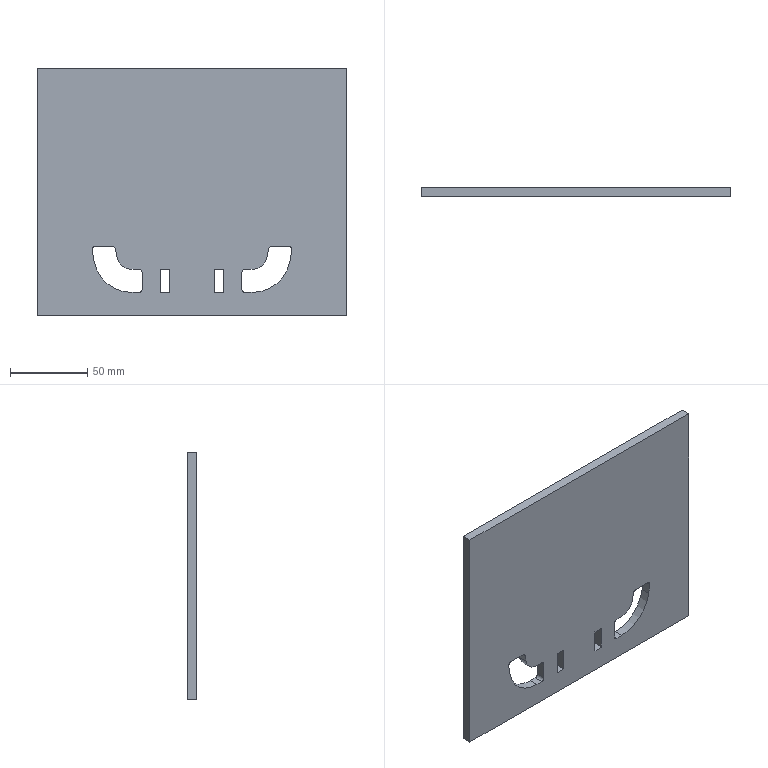Part | SolidWorks | features Cut 1, FlatPattern 1, ICE 1, SMBaseFlange 1, SheetMetal 1 | 1 solid | 38 faces | box 200 x 6 x 160 mm | volume 183961 mm3 | plane 26 | cylinder 12 | commonest cylinder face diameters 4 x8 20 x2 50 x2
STEP:
#1=CARTESIAN_POINT('',(100.,0.,80.));
#2=VERTEX_POINT('',#1);
#3=CARTESIAN_POINT('',(100.,0.,-80.));
#4=VERTEX_POINT('',#3);
#5=CARTESIAN_POINT('',(100.,0.,-80.));
#6=DIRECTION('',(0.,0.,-1.));
#7=VECTOR('',#6,1000.);
#8=LINE('',#5,#7);
#9=EDGE_CURVE('',#2,#4,#8,.T.);
#10=ORIENTED_EDGE('',*,*,#9,.T.);
#11=CARTESIAN_POINT('',(100.,6.,-80.));
#12=VERTEX_POINT('',#11);
#13=CARTESIAN_POINT('',(100.,6.,-80.));
#14=DIRECTION('',(0.,-1.,0.));
#15=VECTOR('',#14,1000.);
#16=LINE('',#13,#15);
#17=EDGE_CURVE('',#12,#4,#16,.T.);
#18=ORIENTED_EDGE('',*,*,#17,.F.);
#19=CARTESIAN_POINT('',(100.,6.,80.));
#20=VERTEX_POINT('',#19);
#21=CARTESIAN_POINT('',(100.,6.,-80.));
#22=DIRECTION('',(0.,0.,-1.));
#23=VECTOR('',#22,1000.);
#24=LINE('',#21,#23);
#25=EDGE_CURVE('',#20,#12,#24,.T.);
#26=ORIENTED_EDGE('',*,*,#25,.F.);
#27=CARTESIAN_POINT('',(100.,6.,80.));
#28=DIRECTION('',(0.,-1.,0.));
#29=VECTOR('',#28,1000.);
#30=LINE('',#27,#29);
#31=EDGE_CURVE('',#20,#2,#30,.T.);
#32=ORIENTED_EDGE('',*,*,#31,.T.);
#33=EDGE_LOOP('',(#10,#18,#26,#32));
#34=FACE_OUTER_BOUND('',#33,.T.);
#35=CARTESIAN_POINT('',(100.,6.,-80.));
#36=DIRECTION('',(-1.,0.,0.));
#37=DIRECTION('',(0.,0.,1.));
#38=AXIS2_PLACEMENT_3D('',#35,#36,#37);
#39=PLANE('',#38);
#40=ADVANCED_FACE('',(#34),#39,.F.);
#41=CARTESIAN_POINT('',(-100.,0.,-80.));
#42=VERTEX_POINT('',#41);
#43=CARTESIAN_POINT('',(-100.,0.,-80.));
#44=DIRECTION('',(-1.,0.,0.));
#45=VECTOR('',#44,1000.);
#46=LINE('',#43,#45);
#47=EDGE_CURVE('',#4,#42,#46,.T.);
#48=ORIENTED_EDGE('',*,*,#47,.T.);
#49=CARTESIAN_POINT('',(-100.,6.,-80.));
#50=VERTEX_POINT('',#49);
#51=CARTESIAN_POINT('',(-100.,6.,-80.));
#52=DIRECTION('',(0.,-1.,0.));
#53=VECTOR('',#52,1000.);
#54=LINE('',#51,#53);
#55=EDGE_CURVE('',#50,#42,#54,.T.);
#56=ORIENTED_EDGE('',*,*,#55,.F.);
#57=CARTESIAN_POINT('',(-100.,6.,-80.));
#58=DIRECTION('',(-1.,0.,0.));
#59=VECTOR('',#58,1000.);
#60=LINE('',#57,#59);
#61=EDGE_CURVE('',#12,#50,#60,.T.);
#62=ORIENTED_EDGE('',*,*,#61,.F.);
#63=ORIENTED_EDGE('',*,*,#17,.T.);
#64=EDGE_LOOP('',(#48,#56,#62,#63));
#65=FACE_OUTER_BOUND('',#64,.T.);
#66=CARTESIAN_POINT('',(-100.,6.,-80.));
#67=DIRECTION('',(0.,0.,1.));
#68=DIRECTION('',(1.,0.,0.));
#69=AXIS2_PLACEMENT_3D('',#66,#67,#68);
#70=PLANE('',#69);
#71=ADVANCED_FACE('',(#65),#70,.F.);
#72=CARTESIAN_POINT('',(-100.,0.,80.));
#73=VERTEX_POINT('',#72);
#74=CARTESIAN_POINT('',(-100.,0.,-80.));
#75=DIRECTION('',(0.,0.,1.));
#76=VECTOR('',#75,1000.);
#77=LINE('',#74,#76);
#78=EDGE_CURVE('',#42,#73,#77,.T.);
#79=ORIENTED_EDGE('',*,*,#78,.T.);
#80=CARTESIAN_POINT('',(-100.,6.,80.));
#81=VERTEX_POINT('',#80);
#82=CARTESIAN_POINT('',(-100.,6.,80.));
#83=DIRECTION('',(0.,-1.,0.));
#84=VECTOR('',#83,1000.);
#85=LINE('',#82,#84);
#86=EDGE_CURVE('',#81,#73,#85,.T.);
#87=ORIENTED_EDGE('',*,*,#86,.F.);
#88=CARTESIAN_POINT('',(-100.,6.,-80.));
#89=DIRECTION('',(0.,0.,1.));
#90=VECTOR('',#89,1000.);
#91=LINE('',#88,#90);
#92=EDGE_CURVE('',#50,#81,#91,.T.);
#93=ORIENTED_EDGE('',*,*,#92,.F.);
#94=ORIENTED_EDGE('',*,*,#55,.T.);
#95=EDGE_LOOP('',(#79,#87,#93,#94));
#96=FACE_OUTER_BOUND('',#95,.T.);
#97=CARTESIAN_POINT('',(-100.,6.,-80.));
#98=DIRECTION('',(1.,0.,0.));
#99=DIRECTION('',(0.,0.,-1.));
#100=AXIS2_PLACEMENT_3D('',#97,#98,#99);
#101=PLANE('',#100);
#102=ADVANCED_FACE('',(#96),#101,.F.);
#103=CARTESIAN_POINT('',(-100.,0.,80.));
#104=DIRECTION('',(1.,0.,0.));
#105=VECTOR('',#104,1000.);
#106=LINE('',#103,#105);
#107=EDGE_CURVE('',#73,#2,#106,.T.);
#108=ORIENTED_EDGE('',*,*,#107,.T.);
#109=ORIENTED_EDGE('',*,*,#31,.F.);
#110=CARTESIAN_POINT('',(-100.,6.,80.));
#111=DIRECTION('',(1.,0.,0.));
#112=VECTOR('',#111,1000.);
#113=LINE('',#110,#112);
#114=EDGE_CURVE('',#81,#20,#113,.T.);
#115=ORIENTED_EDGE('',*,*,#114,.F.);
#116=ORIENTED_EDGE('',*,*,#86,.T.);
#117=EDGE_LOOP('',(#108,#109,#115,#116));
#118=FACE_OUTER_BOUND('',#117,.T.);
#119=CARTESIAN_POINT('',(-100.,6.,80.));
#120=DIRECTION('',(0.,0.,-1.));
#121=DIRECTION('',(-1.,0.,0.));
#122=AXIS2_PLACEMENT_3D('',#119,#120,#121);
#123=PLANE('',#122);
#124=ADVANCED_FACE('',(#118),#123,.F.);
#125=CARTESIAN_POINT('',(-14.299,6.,-50.));
#126=VERTEX_POINT('',#125);
#127=CARTESIAN_POINT('',(-14.299,6.,-65.));
#128=VERTEX_POINT('',#127);
#129=CARTESIAN_POINT('',(-14.299,6.,-65.));
#130=DIRECTION('',(0.,0.,-1.));
#131=VECTOR('',#130,1000.);
#132=LINE('',#129,#131);
#133=EDGE_CURVE('',#126,#128,#132,.T.);
#134=ORIENTED_EDGE('',*,*,#133,.F.);
#135=CARTESIAN_POINT('',(-20.299,6.,-50.));
#136=VERTEX_POINT('',#135);
#137=CARTESIAN_POINT('',(-20.299,6.,-50.));
#138=DIRECTION('',(1.,0.,0.));
#139=VECTOR('',#138,1000.);
#140=LINE('',#137,#139);
#141=EDGE_CURVE('',#136,#126,#140,.T.);
#142=ORIENTED_EDGE('',*,*,#141,.F.);
#143=CARTESIAN_POINT('',(-20.299,6.,-65.));
#144=VERTEX_POINT('',#143);
#145=CARTESIAN_POINT('',(-20.299,6.,-65.));
#146=DIRECTION('',(0.,0.,1.));
#147=VECTOR('',#146,1000.);
#148=LINE('',#145,#147);
#149=EDGE_CURVE('',#144,#136,#148,.T.);
#150=ORIENTED_EDGE('',*,*,#149,.F.);
#151=CARTESIAN_POINT('',(-20.299,6.,-65.));
#152=DIRECTION('',(-1.,0.,0.));
#153=VECTOR('',#152,1000.);
#154=LINE('',#151,#153);
#155=EDGE_CURVE('',#128,#144,#154,.T.);
#156=ORIENTED_EDGE('',*,*,#155,.F.);
#157=EDGE_LOOP('',(#134,#142,#150,#156));
#158=FACE_BOUND('',#157,.T.);
#159=CARTESIAN_POINT('',(20.299,6.,-50.));
#160=VERTEX_POINT('',#159);
#161=CARTESIAN_POINT('',(20.299,6.,-65.));
#162=VERTEX_POINT('',#161);
#163=CARTESIAN_POINT('',(20.299,6.,-65.));
#164=DIRECTION('',(0.,0.,-1.));
#165=VECTOR('',#164,1000.);
#166=LINE('',#163,#165);
#167=EDGE_CURVE('',#160,#162,#166,.T.);
#168=ORIENTED_EDGE('',*,*,#167,.F.);
#169=CARTESIAN_POINT('',(14.299,6.,-50.));
#170=VERTEX_POINT('',#169);
#171=CARTESIAN_POINT('',(20.299,6.,-50.));
#172=DIRECTION('',(1.,0.,0.));
#173=VECTOR('',#172,1000.);
#174=LINE('',#171,#173);
#175=EDGE_CURVE('',#170,#160,#174,.T.);
#176=ORIENTED_EDGE('',*,*,#175,.F.);
#177=CARTESIAN_POINT('',(14.299,6.,-65.));
#178=VERTEX_POINT('',#177);
#179=CARTESIAN_POINT('',(14.299,6.,-65.));
#180=DIRECTION('',(0.,0.,1.));
#181=VECTOR('',#180,1000.);
#182=LINE('',#179,#181);
#183=EDGE_CURVE('',#178,#170,#182,.T.);
#184=ORIENTED_EDGE('',*,*,#183,.F.);
#185=CARTESIAN_POINT('',(20.299,6.,-65.));
#186=DIRECTION('',(-1.,0.,0.));
#187=VECTOR('',#186,1000.);
#188=LINE('',#185,#187);
#189=EDGE_CURVE('',#162,#178,#188,.T.);
#190=ORIENTED_EDGE('',*,*,#189,.F.);
#191=EDGE_LOOP('',(#168,#176,#184,#190));
#192=FACE_BOUND('',#191,.T.);
#193=CARTESIAN_POINT('',(-38.819,6.,-65.));
#194=VERTEX_POINT('',#193);
#195=CARTESIAN_POINT('',(-63.483,6.,-44.083));
#196=VERTEX_POINT('',#195);
#197=CARTESIAN_POINT('',(-38.819,6.,-40.));
#198=DIRECTION('',(0.,1.,0.));
#199=DIRECTION('',(0.,0.,1.));
#200=AXIS2_PLACEMENT_3D('',#197,#198,#199);
#201=CIRCLE('',#200,25.);
#202=EDGE_CURVE('',#194,#196,#201,.T.);
#203=ORIENTED_EDGE('',*,*,#202,.F.);
#204=CARTESIAN_POINT('',(-34.299,6.,-65.));
#205=VERTEX_POINT('',#204);
#206=CARTESIAN_POINT('',(-34.299,6.,-65.));
#207=DIRECTION('',(-1.,0.,0.));
#208=VECTOR('',#207,1000.);
#209=LINE('',#206,#208);
#210=EDGE_CURVE('',#205,#194,#209,.T.);
#211=ORIENTED_EDGE('',*,*,#210,.F.);
#212=CARTESIAN_POINT('',(-32.299,6.,-63.));
#213=VERTEX_POINT('',#212);
#214=CARTESIAN_POINT('',(-34.299,6.,-63.));
#215=DIRECTION('',(0.,1.,0.));
#216=DIRECTION('',(0.,0.,1.));
#217=AXIS2_PLACEMENT_3D('',#214,#215,#216);
#218=CIRCLE('',#217,2.);
#219=EDGE_CURVE('',#213,#205,#218,.T.);
#220=ORIENTED_EDGE('',*,*,#219,.F.);
#221=CARTESIAN_POINT('',(-32.299,6.,-52.));
#222=VERTEX_POINT('',#221);
#223=CARTESIAN_POINT('',(-32.299,6.,-52.));
#224=DIRECTION('',(0.,0.,-1.));
#225=VECTOR('',#224,1000.);
#226=LINE('',#223,#225);
#227=EDGE_CURVE('',#222,#213,#226,.T.);
#228=ORIENTED_EDGE('',*,*,#227,.F.);
#229=CARTESIAN_POINT('',(-34.299,6.,-50.));
#230=VERTEX_POINT('',#229);
#231=CARTESIAN_POINT('',(-34.299,6.,-52.));
#232=DIRECTION('',(0.,1.,0.));
#233=DIRECTION('',(0.,0.,1.));
#234=AXIS2_PLACEMENT_3D('',#231,#232,#233);
#235=CIRCLE('',#234,2.);
#236=EDGE_CURVE('',#230,#222,#235,.T.);
#237=ORIENTED_EDGE('',*,*,#236,.F.);
#238=CARTESIAN_POINT('',(-38.819,6.,-50.));
#239=VERTEX_POINT('',#238);
#240=CARTESIAN_POINT('',(-38.819,6.,-50.));
#241=DIRECTION('',(1.,0.,0.));
#242=VECTOR('',#241,1000.);
#243=LINE('',#240,#242);
#244=EDGE_CURVE('',#239,#230,#243,.T.);
#245=ORIENTED_EDGE('',*,*,#244,.F.);
#246=CARTESIAN_POINT('',(-48.685,6.,-41.633));
#247=VERTEX_POINT('',#246);
#248=CARTESIAN_POINT('',(-38.819,6.,-40.));
#249=DIRECTION('',(0.,-1.,0.));
#250=DIRECTION('',(0.,0.,1.));
#251=AXIS2_PLACEMENT_3D('',#248,#249,#250);
#252=CIRCLE('',#251,10.);
#253=EDGE_CURVE('',#247,#239,#252,.T.);
#254=ORIENTED_EDGE('',*,*,#253,.F.);
#255=CARTESIAN_POINT('',(-49.472,6.,-36.875));
#256=VERTEX_POINT('',#255);
#257=CARTESIAN_POINT('',(-49.472,6.,-36.875));
#258=DIRECTION('',(0.1633,0.,-0.9866));
#259=VECTOR('',#258,1000.);
#260=LINE('',#257,#259);
#261=EDGE_CURVE('',#256,#247,#260,.T.);
#262=ORIENTED_EDGE('',*,*,#261,.F.);
#263=CARTESIAN_POINT('',(-51.446,6.,-35.201));
#264=VERTEX_POINT('',#263);
#265=CARTESIAN_POINT('',(-51.446,6.,-37.201));
#266=DIRECTION('',(0.,1.,0.));
#267=DIRECTION('',(0.,0.,1.));
#268=AXIS2_PLACEMENT_3D('',#265,#266,#267);
#269=CIRCLE('',#268,2.);
#270=EDGE_CURVE('',#264,#256,#269,.T.);
#271=ORIENTED_EDGE('',*,*,#270,.F.);
#272=CARTESIAN_POINT('',(-62.595,6.,-35.201));
#273=VERTEX_POINT('',#272);
#274=CARTESIAN_POINT('',(-62.595,6.,-35.201));
#275=DIRECTION('',(1.,0.,0.));
#276=VECTOR('',#275,1000.);
#277=LINE('',#274,#276);
#278=EDGE_CURVE('',#273,#264,#277,.T.);
#279=ORIENTED_EDGE('',*,*,#278,.F.);
#280=CARTESIAN_POINT('',(-64.568,6.,-37.528));
#281=VERTEX_POINT('',#280);
#282=CARTESIAN_POINT('',(-62.595,6.,-37.201));
#283=DIRECTION('',(0.,1.,0.));
#284=DIRECTION('',(0.,0.,1.));
#285=AXIS2_PLACEMENT_3D('',#282,#283,#284);
#286=CIRCLE('',#285,2.);
#287=EDGE_CURVE('',#281,#273,#286,.T.);
#288=ORIENTED_EDGE('',*,*,#287,.F.);
#289=CARTESIAN_POINT('',(-63.483,6.,-44.083));
#290=DIRECTION('',(-0.1633,0.,0.9866));
#291=VECTOR('',#290,1000.);
#292=LINE('',#289,#291);
#293=EDGE_CURVE('',#196,#281,#292,.T.);
#294=ORIENTED_EDGE('',*,*,#293,.F.);
#295=EDGE_LOOP('',(#203,#211,#220,#228,#237,#245,#254,#262,#271,#279,#288,#294));
#296=FACE_BOUND('',#295,.T.);
#297=CARTESIAN_POINT('',(49.472,6.,-36.875));
#298=VERTEX_POINT('',#297);
#299=CARTESIAN_POINT('',(51.446,6.,-35.201));
#300=VERTEX_POINT('',#299);
#301=CARTESIAN_POINT('',(51.446,6.,-37.201));
#302=DIRECTION('',(0.,1.,0.));
#303=DIRECTION('',(0.,0.,1.));
#304=AXIS2_PLACEMENT_3D('',#301,#302,#303);
#305=CIRCLE('',#304,2.);
#306=EDGE_CURVE('',#298,#300,#305,.T.);
#307=ORIENTED_EDGE('',*,*,#306,.F.);
#308=CARTESIAN_POINT('',(48.685,6.,-41.633));
#309=VERTEX_POINT('',#308);
#310=CARTESIAN_POINT('',(48.685,6.,-41.633));
#311=DIRECTION('',(0.1633,0.,0.9866));
#312=VECTOR('',#311,1000.);
#313=LINE('',#310,#312);
#314=EDGE_CURVE('',#309,#298,#313,.T.);
#315=ORIENTED_EDGE('',*,*,#314,.F.);
#316=CARTESIAN_POINT('',(38.819,6.,-50.));
#317=VERTEX_POINT('',#316);
#318=CARTESIAN_POINT('',(38.819,6.,-40.));
#319=DIRECTION('',(0.,-1.,0.));
#320=DIRECTION('',(0.,0.,1.));
#321=AXIS2_PLACEMENT_3D('',#318,#319,#320);
#322=CIRCLE('',#321,10.);
#323=EDGE_CURVE('',#317,#309,#322,.T.);
#324=ORIENTED_EDGE('',*,*,#323,.F.);
#325=CARTESIAN_POINT('',(34.299,6.,-50.));
#326=VERTEX_POINT('',#325);
#327=CARTESIAN_POINT('',(34.299,6.,-50.));
#328=DIRECTION('',(1.,0.,0.));
#329=VECTOR('',#328,1000.);
#330=LINE('',#327,#329);
#331=EDGE_CURVE('',#326,#317,#330,.T.);
#332=ORIENTED_EDGE('',*,*,#331,.F.);
#333=CARTESIAN_POINT('',(32.299,6.,-52.));
#334=VERTEX_POINT('',#333);
#335=CARTESIAN_POINT('',(34.299,6.,-52.));
#336=DIRECTION('',(0.,1.,0.));
#337=DIRECTION('',(0.,0.,1.));
#338=AXIS2_PLACEMENT_3D('',#335,#336,#337);
#339=CIRCLE('',#338,2.);
#340=EDGE_CURVE('',#334,#326,#339,.T.);
#341=ORIENTED_EDGE('',*,*,#340,.F.);
#342=CARTESIAN_POINT('',(32.299,6.,-63.));
#343=VERTEX_POINT('',#342);
#344=CARTESIAN_POINT('',(32.299,6.,-63.));
#345=DIRECTION('',(0.,0.,1.));
#346=VECTOR('',#345,1000.);
#347=LINE('',#344,#346);
#348=EDGE_CURVE('',#343,#334,#347,.T.);
#349=ORIENTED_EDGE('',*,*,#348,.F.);
#350=CARTESIAN_POINT('',(34.299,6.,-65.));
#351=VERTEX_POINT('',#350);
#352=CARTESIAN_POINT('',(34.299,6.,-63.));
#353=DIRECTION('',(0.,1.,0.));
#354=DIRECTION('',(0.,0.,1.));
#355=AXIS2_PLACEMENT_3D('',#352,#353,#354);
#356=CIRCLE('',#355,2.);
#357=EDGE_CURVE('',#351,#343,#356,.T.);
#358=ORIENTED_EDGE('',*,*,#357,.F.);
#359=CARTESIAN_POINT('',(38.819,6.,-65.));
#360=VERTEX_POINT('',#359);
#361=CARTESIAN_POINT('',(38.819,6.,-65.));
#362=DIRECTION('',(-1.,0.,0.));
#363=VECTOR('',#362,1000.);
#364=LINE('',#361,#363);
#365=EDGE_CURVE('',#360,#351,#364,.T.);
#366=ORIENTED_EDGE('',*,*,#365,.F.);
#367=CARTESIAN_POINT('',(63.483,6.,-44.083));
#368=VERTEX_POINT('',#367);
#369=CARTESIAN_POINT('',(38.819,6.,-40.));
#370=DIRECTION('',(0.,1.,0.));
#371=DIRECTION('',(0.,0.,1.));
#372=AXIS2_PLACEMENT_3D('',#369,#370,#371);
#373=CIRCLE('',#372,25.);
#374=EDGE_CURVE('',#368,#360,#373,.T.);
#375=ORIENTED_EDGE('',*,*,#374,.F.);
#376=CARTESIAN_POINT('',(64.568,6.,-37.528));
#377=VERTEX_POINT('',#376);
#378=CARTESIAN_POINT('',(64.568,6.,-37.528));
#379=DIRECTION('',(-0.1633,0.,-0.9866));
#380=VECTOR('',#379,1000.);
#381=LINE('',#378,#380);
#382=EDGE_CURVE('',#377,#368,#381,.T.);
#383=ORIENTED_EDGE('',*,*,#382,.F.);
#384=CARTESIAN_POINT('',(62.595,6.,-35.201));
#385=VERTEX_POINT('',#384);
#386=CARTESIAN_POINT('',(62.595,6.,-37.201));
#387=DIRECTION('',(0.,1.,0.));
#388=DIRECTION('',(0.,0.,1.));
#389=AXIS2_PLACEMENT_3D('',#386,#387,#388);
#390=CIRCLE('',#389,2.);
#391=EDGE_CURVE('',#385,#377,#390,.T.);
#392=ORIENTED_EDGE('',*,*,#391,.F.);
#393=CARTESIAN_POINT('',(51.446,6.,-35.201));
#394=DIRECTION('',(1.,0.,0.));
#395=VECTOR('',#394,1000.);
#396=LINE('',#393,#395);
#397=EDGE_CURVE('',#300,#385,#396,.T.);
#398=ORIENTED_EDGE('',*,*,#397,.F.);
#399=EDGE_LOOP('',(#307,#315,#324,#332,#341,#349,#358,#366,#375,#383,#392,#398));
#400=FACE_BOUND('',#399,.T.);
#401=ORIENTED_EDGE('',*,*,#25,.T.);
#402=ORIENTED_EDGE('',*,*,#61,.T.);
#403=ORIENTED_EDGE('',*,*,#92,.T.);
#404=ORIENTED_EDGE('',*,*,#114,.T.);
#405=EDGE_LOOP('',(#401,#402,#403,#404));
#406=FACE_OUTER_BOUND('',#405,.T.);
#407=CARTESIAN_POINT('',(0.,6.,0.));
#408=DIRECTION('',(0.,1.,0.));
#409=DIRECTION('',(0.,0.,1.));
#410=AXIS2_PLACEMENT_3D('',#407,#408,#409);
#411=PLANE('',#410);
#412=ADVANCED_FACE('',(#158,#192,#296,#400,#406),#411,.T.);
#413=CARTESIAN_POINT('',(-20.299,0.,-50.));
#414=VERTEX_POINT('',#413);
#415=CARTESIAN_POINT('',(-14.299,0.,-50.));
#416=VERTEX_POINT('',#415);
#417=CARTESIAN_POINT('',(-20.299,0.,-50.));
#418=DIRECTION('',(1.,0.,0.));
#419=VECTOR('',#418,1000.);
#420=LINE('',#417,#419);
#421=EDGE_CURVE('',#414,#416,#420,.T.);
#422=ORIENTED_EDGE('',*,*,#421,.T.);
#423=CARTESIAN_POINT('',(-14.299,0.,-65.));
#424=VERTEX_POINT('',#423);
#425=CARTESIAN_POINT('',(-14.299,0.,-65.));
#426=DIRECTION('',(0.,0.,-1.));
#427=VECTOR('',#426,1000.);
#428=LINE('',#425,#427);
#429=EDGE_CURVE('',#416,#424,#428,.T.);
#430=ORIENTED_EDGE('',*,*,#429,.T.);
#431=CARTESIAN_POINT('',(-20.299,0.,-65.));
#432=VERTEX_POINT('',#431);
#433=CARTESIAN_POINT('',(-20.299,0.,-65.));
#434=DIRECTION('',(-1.,0.,0.));
#435=VECTOR('',#434,1000.);
#436=LINE('',#433,#435);
#437=EDGE_CURVE('',#424,#432,#436,.T.);
#438=ORIENTED_EDGE('',*,*,#437,.T.);
#439=CARTESIAN_POINT('',(-20.299,0.,-65.));
#440=DIRECTION('',(0.,0.,1.));
#441=VECTOR('',#440,1000.);
#442=LINE('',#439,#441);
#443=EDGE_CURVE('',#432,#414,#442,.T.);
#444=ORIENTED_EDGE('',*,*,#443,.T.);
#445=EDGE_LOOP('',(#422,#430,#438,#444));
#446=FACE_BOUND('',#445,.T.);
#447=CARTESIAN_POINT('',(14.299,0.,-50.));
#448=VERTEX_POINT('',#447);
#449=CARTESIAN_POINT('',(20.299,0.,-50.));
#450=VERTEX_POINT('',#449);
#451=CARTESIAN_POINT('',(20.299,0.,-50.));
#452=DIRECTION('',(1.,0.,0.));
#453=VECTOR('',#452,1000.);
#454=LINE('',#451,#453);
#455=EDGE_CURVE('',#448,#450,#454,.T.);
#456=ORIENTED_EDGE('',*,*,#455,.T.);
#457=CARTESIAN_POINT('',(20.299,0.,-65.));
#458=VERTEX_POINT('',#457);
#459=CARTESIAN_POINT('',(20.299,0.,-65.));
#460=DIRECTION('',(0.,0.,-1.));
#461=VECTOR('',#460,1000.);
#462=LINE('',#459,#461);
#463=EDGE_CURVE('',#450,#458,#462,.T.);
#464=ORIENTED_EDGE('',*,*,#463,.T.);
#465=CARTESIAN_POINT('',(14.299,0.,-65.));
#466=VERTEX_POINT('',#465);
#467=CARTESIAN_POINT('',(20.299,0.,-65.));
#468=DIRECTION('',(-1.,0.,0.));
#469=VECTOR('',#468,1000.);
#470=LINE('',#467,#469);
#471=EDGE_CURVE('',#458,#466,#470,.T.);
#472=ORIENTED_EDGE('',*,*,#471,.T.);
#473=CARTESIAN_POINT('',(14.299,0.,-65.));
#474=DIRECTION('',(0.,0.,1.));
#475=VECTOR('',#474,1000.);
#476=LINE('',#473,#475);
#477=EDGE_CURVE('',#466,#448,#476,.T.);
#478=ORIENTED_EDGE('',*,*,#477,.T.);
#479=EDGE_LOOP('',(#456,#464,#472,#478));
#480=FACE_BOUND('',#479,.T.);
#481=CARTESIAN_POINT('',(-34.299,0.,-65.));
#482=VERTEX_POINT('',#481);
#483=CARTESIAN_POINT('',(-38.819,0.,-65.));
#484=VERTEX_POINT('',#483);
#485=CARTESIAN_POINT('',(-34.299,0.,-65.));
#486=DIRECTION('',(-1.,0.,0.));
#487=VECTOR('',#486,1000.);
#488=LINE('',#485,#487);
#489=EDGE_CURVE('',#482,#484,#488,.T.);
#490=ORIENTED_EDGE('',*,*,#489,.T.);
#491=CARTESIAN_POINT('',(-63.483,0.,-44.083));
#492=VERTEX_POINT('',#491);
#493=CARTESIAN_POINT('',(-38.819,0.,-40.));
#494=DIRECTION('',(0.,1.,0.));
#495=DIRECTION('',(0.,0.,1.));
#496=AXIS2_PLACEMENT_3D('',#493,#494,#495);
#497=CIRCLE('',#496,25.);
#498=EDGE_CURVE('',#484,#492,#497,.T.);
#499=ORIENTED_EDGE('',*,*,#498,.T.);
#500=CARTESIAN_POINT('',(-64.568,0.,-37.528));
#501=VERTEX_POINT('',#500);
#502=CARTESIAN_POINT('',(-63.483,0.,-44.083));
#503=DIRECTION('',(-0.1633,0.,0.9866));
#504=VECTOR('',#503,1000.);
#505=LINE('',#502,#504);
#506=EDGE_CURVE('',#492,#501,#505,.T.);
#507=ORIENTED_EDGE('',*,*,#506,.T.);
#508=CARTESIAN_POINT('',(-62.595,0.,-35.201));
#509=VERTEX_POINT('',#508);
#510=CARTESIAN_POINT('',(-62.595,0.,-37.201));
#511=DIRECTION('',(0.,1.,0.));
#512=DIRECTION('',(0.,0.,1.));
#513=AXIS2_PLACEMENT_3D('',#510,#511,#512);
#514=CIRCLE('',#513,2.);
#515=EDGE_CURVE('',#501,#509,#514,.T.);
#516=ORIENTED_EDGE('',*,*,#515,.T.);
#517=CARTESIAN_POINT('',(-51.446,0.,-35.201));
#518=VERTEX_POINT('',#517);
#519=CARTESIAN_POINT('',(-62.595,0.,-35.201));
#520=DIRECTION('',(1.,0.,0.));
#521=VECTOR('',#520,1000.);
#522=LINE('',#519,#521);
#523=EDGE_CURVE('',#509,#518,#522,.T.);
#524=ORIENTED_EDGE('',*,*,#523,.T.);
#525=CARTESIAN_POINT('',(-49.472,0.,-36.875));
#526=VERTEX_POINT('',#525);
#527=CARTESIAN_POINT('',(-51.446,0.,-37.201));
#528=DIRECTION('',(0.,1.,0.));
#529=DIRECTION('',(0.,0.,1.));
#530=AXIS2_PLACEMENT_3D('',#527,#528,#529);
#531=CIRCLE('',#530,2.);
#532=EDGE_CURVE('',#518,#526,#531,.T.);
#533=ORIENTED_EDGE('',*,*,#532,.T.);
#534=CARTESIAN_POINT('',(-48.685,0.,-41.633));
#535=VERTEX_POINT('',#534);
#536=CARTESIAN_POINT('',(-49.472,0.,-36.875));
#537=DIRECTION('',(0.1633,0.,-0.9866));
#538=VECTOR('',#537,1000.);
#539=LINE('',#536,#538);
#540=EDGE_CURVE('',#526,#535,#539,.T.);
#541=ORIENTED_EDGE('',*,*,#540,.T.);
#542=CARTESIAN_POINT('',(-38.819,0.,-50.));
#543=VERTEX_POINT('',#542);
#544=CARTESIAN_POINT('',(-38.819,0.,-40.));
#545=DIRECTION('',(0.,-1.,0.));
#546=DIRECTION('',(0.,0.,1.));
#547=AXIS2_PLACEMENT_3D('',#544,#545,#546);
#548=CIRCLE('',#547,10.);
#549=EDGE_CURVE('',#535,#543,#548,.T.);
#550=ORIENTED_EDGE('',*,*,#549,.T.);
#551=CARTESIAN_POINT('',(-34.299,0.,-50.));
#552=VERTEX_POINT('',#551);
#553=CARTESIAN_POINT('',(-38.819,0.,-50.));
#554=DIRECTION('',(1.,0.,0.));
#555=VECTOR('',#554,1000.);
#556=LINE('',#553,#555);
#557=EDGE_CURVE('',#543,#552,#556,.T.);
#558=ORIENTED_EDGE('',*,*,#557,.T.);
#559=CARTESIAN_POINT('',(-32.299,0.,-52.));
#560=VERTEX_POINT('',#559);
#561=CARTESIAN_POINT('',(-34.299,0.,-52.));
#562=DIRECTION('',(0.,1.,0.));
#563=DIRECTION('',(0.,0.,1.));
#564=AXIS2_PLACEMENT_3D('',#561,#562,#563);
#565=CIRCLE('',#564,2.);
#566=EDGE_CURVE('',#552,#560,#565,.T.);
#567=ORIENTED_EDGE('',*,*,#566,.T.);
#568=CARTESIAN_POINT('',(-32.299,0.,-63.));
#569=VERTEX_POINT('',#568);
#570=CARTESIAN_POINT('',(-32.299,0.,-52.));
#571=DIRECTION('',(0.,0.,-1.));
#572=VECTOR('',#571,1000.);
#573=LINE('',#570,#572);
#574=EDGE_CURVE('',#560,#569,#573,.T.);
#575=ORIENTED_EDGE('',*,*,#574,.T.);
#576=CARTESIAN_POINT('',(-34.299,0.,-63.));
#577=DIRECTION('',(0.,1.,0.));
#578=DIRECTION('',(0.,0.,1.));
#579=AXIS2_PLACEMENT_3D('',#576,#577,#578);
#580=CIRCLE('',#579,2.);
#581=EDGE_CURVE('',#569,#482,#580,.T.);
#582=ORIENTED_EDGE('',*,*,#581,.T.);
#583=EDGE_LOOP('',(#490,#499,#507,#516,#524,#533,#541,#550,#558,#567,#575,#582));
#584=FACE_BOUND('',#583,.T.);
#585=CARTESIAN_POINT('',(48.685,0.,-41.633));
#586=VERTEX_POINT('',#585);
#587=CARTESIAN_POINT('',(49.472,0.,-36.875));
#588=VERTEX_POINT('',#587);
#589=CARTESIAN_POINT('',(48.685,0.,-41.633));
#590=DIRECTION('',(0.1633,0.,0.9866));
#591=VECTOR('',#590,1000.);
#592=LINE('',#589,#591);
#593=EDGE_CURVE('',#586,#588,#592,.T.);
#594=ORIENTED_EDGE('',*,*,#593,.T.);
#595=CARTESIAN_POINT('',(51.446,0.,-35.201));
#596=VERTEX_POINT('',#595);
#597=CARTESIAN_POINT('',(51.446,0.,-37.201));
#598=DIRECTION('',(0.,1.,0.));
#599=DIRECTION('',(0.,0.,1.));
#600=AXIS2_PLACEMENT_3D('',#597,#598,#599);
#601=CIRCLE('',#600,2.);
#602=EDGE_CURVE('',#588,#596,#601,.T.);
#603=ORIENTED_EDGE('',*,*,#602,.T.);
#604=CARTESIAN_POINT('',(62.595,0.,-35.201));
#605=VERTEX_POINT('',#604);
#606=CARTESIAN_POINT('',(51.446,0.,-35.201));
#607=DIRECTION('',(1.,0.,0.));
#608=VECTOR('',#607,1000.);
#609=LINE('',#606,#608);
#610=EDGE_CURVE('',#596,#605,#609,.T.);
#611=ORIENTED_EDGE('',*,*,#610,.T.);
#612=CARTESIAN_POINT('',(64.568,0.,-37.528));
#613=VERTEX_POINT('',#612);
#614=CARTESIAN_POINT('',(62.595,0.,-37.201));
#615=DIRECTION('',(0.,1.,0.));
#616=DIRECTION('',(0.,0.,1.));
#617=AXIS2_PLACEMENT_3D('',#614,#615,#616);
#618=CIRCLE('',#617,2.);
#619=EDGE_CURVE('',#605,#613,#618,.T.);
#620=ORIENTED_EDGE('',*,*,#619,.T.);
#621=CARTESIAN_POINT('',(63.483,0.,-44.083));
#622=VERTEX_POINT('',#621);
#623=CARTESIAN_POINT('',(64.568,0.,-37.528));
#624=DIRECTION('',(-0.1633,0.,-0.9866));
#625=VECTOR('',#624,1000.);
#626=LINE('',#623,#625);
#627=EDGE_CURVE('',#613,#622,#626,.T.);
#628=ORIENTED_EDGE('',*,*,#627,.T.);
#629=CARTESIAN_POINT('',(38.819,0.,-65.));
#630=VERTEX_POINT('',#629);
#631=CARTESIAN_POINT('',(38.819,0.,-40.));
#632=DIRECTION('',(0.,1.,0.));
#633=DIRECTION('',(0.,0.,1.));
#634=AXIS2_PLACEMENT_3D('',#631,#632,#633);
#635=CIRCLE('',#634,25.);
#636=EDGE_CURVE('',#622,#630,#635,.T.);
#637=ORIENTED_EDGE('',*,*,#636,.T.);
#638=CARTESIAN_POINT('',(34.299,0.,-65.));
#639=VERTEX_POINT('',#638);
#640=CARTESIAN_POINT('',(38.819,0.,-65.));
#641=DIRECTION('',(-1.,0.,0.));
#642=VECTOR('',#641,1000.);
#643=LINE('',#640,#642);
#644=EDGE_CURVE('',#630,#639,#643,.T.);
#645=ORIENTED_EDGE('',*,*,#644,.T.);
#646=CARTESIAN_POINT('',(32.299,0.,-63.));
#647=VERTEX_POINT('',#646);
#648=CARTESIAN_POINT('',(34.299,0.,-63.));
#649=DIRECTION('',(0.,1.,0.));
#650=DIRECTION('',(0.,0.,1.));
#651=AXIS2_PLACEMENT_3D('',#648,#649,#650);
#652=CIRCLE('',#651,2.);
#653=EDGE_CURVE('',#639,#647,#652,.T.);
#654=ORIENTED_EDGE('',*,*,#653,.T.);
#655=CARTESIAN_POINT('',(32.299,0.,-52.));
#656=VERTEX_POINT('',#655);
#657=CARTESIAN_POINT('',(32.299,0.,-63.));
#658=DIRECTION('',(0.,0.,1.));
#659=VECTOR('',#658,1000.);
#660=LINE('',#657,#659);
#661=EDGE_CURVE('',#647,#656,#660,.T.);
#662=ORIENTED_EDGE('',*,*,#661,.T.);
#663=CARTESIAN_POINT('',(34.299,0.,-50.));
#664=VERTEX_POINT('',#663);
#665=CARTESIAN_POINT('',(34.299,0.,-52.));
#666=DIRECTION('',(0.,1.,0.));
#667=DIRECTION('',(0.,0.,1.));
#668=AXIS2_PLACEMENT_3D('',#665,#666,#667);
#669=CIRCLE('',#668,2.);
#670=EDGE_CURVE('',#656,#664,#669,.T.);
#671=ORIENTED_EDGE('',*,*,#670,.T.);
#672=CARTESIAN_POINT('',(38.819,0.,-50.));
#673=VERTEX_POINT('',#672);
#674=CARTESIAN_POINT('',(34.299,0.,-50.));
#675=DIRECTION('',(1.,0.,0.));
#676=VECTOR('',#675,1000.);
#677=LINE('',#674,#676);
#678=EDGE_CURVE('',#664,#673,#677,.T.);
#679=ORIENTED_EDGE('',*,*,#678,.T.);
#680=CARTESIAN_POINT('',(38.819,0.,-40.));
#681=DIRECTION('',(0.,-1.,0.));
#682=DIRECTION('',(0.,0.,1.));
#683=AXIS2_PLACEMENT_3D('',#680,#681,#682);
#684=CIRCLE('',#683,10.);
#685=EDGE_CURVE('',#673,#586,#684,.T.);
#686=ORIENTED_EDGE('',*,*,#685,.T.);
#687=EDGE_LOOP('',(#594,#603,#611,#620,#628,#637,#645,#654,#662,#671,#679,#686));
#688=FACE_BOUND('',#687,.T.);
#689=ORIENTED_EDGE('',*,*,#9,.F.);
#690=ORIENTED_EDGE('',*,*,#107,.F.);
#691=ORIENTED_EDGE('',*,*,#78,.F.);
#692=ORIENTED_EDGE('',*,*,#47,.F.);
#693=EDGE_LOOP('',(#689,#690,#691,#692));
#694=FACE_OUTER_BOUND('',#693,.T.);
#695=CARTESIAN_POINT('',(0.,0.,0.));
#696=DIRECTION('',(0.,1.,0.));
#697=DIRECTION('',(0.,0.,1.));
#698=AXIS2_PLACEMENT_3D('',#695,#696,#697);
#699=PLANE('',#698);
#700=ADVANCED_FACE('',(#446,#480,#584,#688,#694),#699,.F.);
#701=ORIENTED_EDGE('',*,*,#306,.T.);
#702=CARTESIAN_POINT('',(51.446,0.,-35.201));
#703=DIRECTION('',(0.,1.,0.));
#704=VECTOR('',#703,1000.);
#705=LINE('',#702,#704);
#706=EDGE_CURVE('',#596,#300,#705,.T.);
#707=ORIENTED_EDGE('',*,*,#706,.F.);
#708=ORIENTED_EDGE('',*,*,#602,.F.);
#709=CARTESIAN_POINT('',(49.472,0.,-36.875));
#710=DIRECTION('',(0.,1.,0.));
#711=VECTOR('',#710,1000.);
#712=LINE('',#709,#711);
#713=EDGE_CURVE('',#588,#298,#712,.T.);
#714=ORIENTED_EDGE('',*,*,#713,.T.);
#715=EDGE_LOOP('',(#701,#707,#708,#714));
#716=FACE_OUTER_BOUND('',#715,.T.);
#717=CARTESIAN_POINT('',(51.446,0.,-37.201));
#718=DIRECTION('',(0.,1.,0.));
#719=DIRECTION('',(0.,0.,1.));
#720=AXIS2_PLACEMENT_3D('',#717,#718,#719);
#721=CYLINDRICAL_SURFACE('',#720,2.);
#722=ADVANCED_FACE('',(#716),#721,.F.);
#723=ORIENTED_EDGE('',*,*,#314,.T.);
#724=ORIENTED_EDGE('',*,*,#713,.F.);
#725=ORIENTED_EDGE('',*,*,#593,.F.);
#726=CARTESIAN_POINT('',(48.685,0.,-41.633));
#727=DIRECTION('',(0.,1.,0.));
#728=VECTOR('',#727,1000.);
#729=LINE('',#726,#728);
#730=EDGE_CURVE('',#586,#309,#729,.T.);
#731=ORIENTED_EDGE('',*,*,#730,.T.);
#732=EDGE_LOOP('',(#723,#724,#725,#731));
#733=FACE_OUTER_BOUND('',#732,.T.);
#734=CARTESIAN_POINT('',(48.685,0.,-41.633));
#735=DIRECTION('',(-0.9866,0.,0.1633));
#736=DIRECTION('',(0.1633,0.,0.9866));
#737=AXIS2_PLACEMENT_3D('',#734,#735,#736);
#738=PLANE('',#737);
#739=ADVANCED_FACE('',(#733),#738,.F.);
#740=ORIENTED_EDGE('',*,*,#323,.T.);
#741=ORIENTED_EDGE('',*,*,#730,.F.);
#742=ORIENTED_EDGE('',*,*,#685,.F.);
#743=CARTESIAN_POINT('',(38.819,0.,-50.));
#744=DIRECTION('',(0.,1.,0.));
#745=VECTOR('',#744,1000.);
#746=LINE('',#743,#745);
#747=EDGE_CURVE('',#673,#317,#746,.T.);
#748=ORIENTED_EDGE('',*,*,#747,.T.);
#749=EDGE_LOOP('',(#740,#741,#742,#748));
#750=FACE_OUTER_BOUND('',#749,.T.);
#751=CARTESIAN_POINT('',(38.819,0.,-40.));
#752=DIRECTION('',(0.,1.,0.));
#753=DIRECTION('',(0.,0.,1.));
#754=AXIS2_PLACEMENT_3D('',#751,#752,#753);
#755=CYLINDRICAL_SURFACE('',#754,10.);
#756=ADVANCED_FACE('',(#750),#755,.T.);
#757=ORIENTED_EDGE('',*,*,#331,.T.);
#758=ORIENTED_EDGE('',*,*,#747,.F.);
#759=ORIENTED_EDGE('',*,*,#678,.F.);
#760=CARTESIAN_POINT('',(34.299,0.,-50.));
#761=DIRECTION('',(0.,1.,0.));
#762=VECTOR('',#761,1000.);
#763=LINE('',#760,#762);
#764=EDGE_CURVE('',#664,#326,#763,.T.);
#765=ORIENTED_EDGE('',*,*,#764,.T.);
#766=EDGE_LOOP('',(#757,#758,#759,#765));
#767=FACE_OUTER_BOUND('',#766,.T.);
#768=CARTESIAN_POINT('',(34.299,0.,-50.));
#769=DIRECTION('',(0.,0.,1.));
#770=DIRECTION('',(1.,0.,0.));
#771=AXIS2_PLACEMENT_3D('',#768,#769,#770);
#772=PLANE('',#771);
#773=ADVANCED_FACE('',(#767),#772,.F.);
#774=ORIENTED_EDGE('',*,*,#340,.T.);
#775=ORIENTED_EDGE('',*,*,#764,.F.);
#776=ORIENTED_EDGE('',*,*,#670,.F.);
#777=CARTESIAN_POINT('',(32.299,0.,-52.));
#778=DIRECTION('',(0.,1.,0.));
#779=VECTOR('',#778,1000.);
#780=LINE('',#777,#779);
#781=EDGE_CURVE('',#656,#334,#780,.T.);
#782=ORIENTED_EDGE('',*,*,#781,.T.);
#783=EDGE_LOOP('',(#774,#775,#776,#782));
#784=FACE_OUTER_BOUND('',#783,.T.);
#785=CARTESIAN_POINT('',(34.299,0.,-52.));
#786=DIRECTION('',(0.,1.,0.));
#787=DIRECTION('',(0.,0.,1.));
#788=AXIS2_PLACEMENT_3D('',#785,#786,#787);
#789=CYLINDRICAL_SURFACE('',#788,2.);
#790=ADVANCED_FACE('',(#784),#789,.F.);
#791=ORIENTED_EDGE('',*,*,#348,.T.);
#792=ORIENTED_EDGE('',*,*,#781,.F.);
#793=ORIENTED_EDGE('',*,*,#661,.F.);
#794=CARTESIAN_POINT('',(32.299,0.,-63.));
#795=DIRECTION('',(0.,1.,0.));
#796=VECTOR('',#795,1000.);
#797=LINE('',#794,#796);
#798=EDGE_CURVE('',#647,#343,#797,.T.);
#799=ORIENTED_EDGE('',*,*,#798,.T.);
#800=EDGE_LOOP('',(#791,#792,#793,#799));
#801=FACE_OUTER_BOUND('',#800,.T.);
#802=CARTESIAN_POINT('',(32.299,0.,-63.));
#803=DIRECTION('',(-1.,0.,0.));
#804=DIRECTION('',(0.,0.,1.));
#805=AXIS2_PLACEMENT_3D('',#802,#803,#804);
#806=PLANE('',#805);
#807=ADVANCED_FACE('',(#801),#806,.F.);
#808=ORIENTED_EDGE('',*,*,#357,.T.);
#809=ORIENTED_EDGE('',*,*,#798,.F.);
#810=ORIENTED_EDGE('',*,*,#653,.F.);
#811=CARTESIAN_POINT('',(34.299,0.,-65.));
#812=DIRECTION('',(0.,1.,0.));
#813=VECTOR('',#812,1000.);
#814=LINE('',#811,#813);
#815=EDGE_CURVE('',#639,#351,#814,.T.);
#816=ORIENTED_EDGE('',*,*,#815,.T.);
#817=EDGE_LOOP('',(#808,#809,#810,#816));
#818=FACE_OUTER_BOUND('',#817,.T.);
#819=CARTESIAN_POINT('',(34.299,0.,-63.));
#820=DIRECTION('',(0.,1.,0.));
#821=DIRECTION('',(0.,0.,1.));
#822=AXIS2_PLACEMENT_3D('',#819,#820,#821);
#823=CYLINDRICAL_SURFACE('',#822,2.);
#824=ADVANCED_FACE('',(#818),#823,.F.);
#825=ORIENTED_EDGE('',*,*,#365,.T.);
#826=ORIENTED_EDGE('',*,*,#815,.F.);
#827=ORIENTED_EDGE('',*,*,#644,.F.);
#828=CARTESIAN_POINT('',(38.819,0.,-65.));
#829=DIRECTION('',(0.,1.,0.));
#830=VECTOR('',#829,1000.);
#831=LINE('',#828,#830);
#832=EDGE_CURVE('',#630,#360,#831,.T.);
#833=ORIENTED_EDGE('',*,*,#832,.T.);
#834=EDGE_LOOP('',(#825,#826,#827,#833));
#835=FACE_OUTER_BOUND('',#834,.T.);
#836=CARTESIAN_POINT('',(38.819,0.,-65.));
#837=DIRECTION('',(0.,0.,-1.));
#838=DIRECTION('',(-1.,0.,0.));
#839=AXIS2_PLACEMENT_3D('',#836,#837,#838);
#840=PLANE('',#839);
#841=ADVANCED_FACE('',(#835),#840,.F.);
#842=ORIENTED_EDGE('',*,*,#374,.T.);
#843=ORIENTED_EDGE('',*,*,#832,.F.);
#844=ORIENTED_EDGE('',*,*,#636,.F.);
#845=CARTESIAN_POINT('',(63.483,0.,-44.083));
#846=DIRECTION('',(0.,1.,0.));
#847=VECTOR('',#846,1000.);
#848=LINE('',#845,#847);
#849=EDGE_CURVE('',#622,#368,#848,.T.);
#850=ORIENTED_EDGE('',*,*,#849,.T.);
#851=EDGE_LOOP('',(#842,#843,#844,#850));
#852=FACE_OUTER_BOUND('',#851,.T.);
#853=CARTESIAN_POINT('',(38.819,0.,-40.));
#854=DIRECTION('',(0.,1.,0.));
#855=DIRECTION('',(0.,0.,1.));
#856=AXIS2_PLACEMENT_3D('',#853,#854,#855);
#857=CYLINDRICAL_SURFACE('',#856,25.);
#858=ADVANCED_FACE('',(#852),#857,.F.);
#859=ORIENTED_EDGE('',*,*,#382,.T.);
#860=ORIENTED_EDGE('',*,*,#849,.F.);
#861=ORIENTED_EDGE('',*,*,#627,.F.);
#862=CARTESIAN_POINT('',(64.568,0.,-37.528));
#863=DIRECTION('',(0.,1.,0.));
#864=VECTOR('',#863,1000.);
#865=LINE('',#862,#864);
#866=EDGE_CURVE('',#613,#377,#865,.T.);
#867=ORIENTED_EDGE('',*,*,#866,.T.);
#868=EDGE_LOOP('',(#859,#860,#861,#867));
#869=FACE_OUTER_BOUND('',#868,.T.);
#870=CARTESIAN_POINT('',(64.568,0.,-37.528));
#871=DIRECTION('',(0.9866,0.,-0.1633));
#872=DIRECTION('',(-0.1633,0.,-0.9866));
#873=AXIS2_PLACEMENT_3D('',#870,#871,#872);
#874=PLANE('',#873);
#875=ADVANCED_FACE('',(#869),#874,.F.);
#876=ORIENTED_EDGE('',*,*,#391,.T.);
#877=ORIENTED_EDGE('',*,*,#866,.F.);
#878=ORIENTED_EDGE('',*,*,#619,.F.);
#879=CARTESIAN_POINT('',(62.595,0.,-35.201));
#880=DIRECTION('',(0.,1.,0.));
#881=VECTOR('',#880,1000.);
#882=LINE('',#879,#881);
#883=EDGE_CURVE('',#605,#385,#882,.T.);
#884=ORIENTED_EDGE('',*,*,#883,.T.);
#885=EDGE_LOOP('',(#876,#877,#878,#884));
#886=FACE_OUTER_BOUND('',#885,.T.);
#887=CARTESIAN_POINT('',(62.595,0.,-37.201));
#888=DIRECTION('',(0.,1.,0.));
#889=DIRECTION('',(0.,0.,1.));
#890=AXIS2_PLACEMENT_3D('',#887,#888,#889);
#891=CYLINDRICAL_SURFACE('',#890,2.);
#892=ADVANCED_FACE('',(#886),#891,.F.);
#893=ORIENTED_EDGE('',*,*,#397,.T.);
#894=ORIENTED_EDGE('',*,*,#883,.F.);
#895=ORIENTED_EDGE('',*,*,#610,.F.);
#896=ORIENTED_EDGE('',*,*,#706,.T.);
#897=EDGE_LOOP('',(#893,#894,#895,#896));
#898=FACE_OUTER_BOUND('',#897,.T.);
#899=CARTESIAN_POINT('',(51.446,0.,-35.201));
#900=DIRECTION('',(0.,0.,1.));
#901=DIRECTION('',(1.,0.,0.));
#902=AXIS2_PLACEMENT_3D('',#899,#900,#901);
#903=PLANE('',#902);
#904=ADVANCED_FACE('',(#898),#903,.F.);
#905=ORIENTED_EDGE('',*,*,#202,.T.);
#906=CARTESIAN_POINT('',(-63.483,0.,-44.083));
#907=DIRECTION('',(0.,1.,0.));
#908=VECTOR('',#907,1000.);
#909=LINE('',#906,#908);
#910=EDGE_CURVE('',#492,#196,#909,.T.);
#911=ORIENTED_EDGE('',*,*,#910,.F.);
#912=ORIENTED_EDGE('',*,*,#498,.F.);
#913=CARTESIAN_POINT('',(-38.819,0.,-65.));
#914=DIRECTION('',(0.,1.,0.));
#915=VECTOR('',#914,1000.);
#916=LINE('',#913,#915);
#917=EDGE_CURVE('',#484,#194,#916,.T.);
#918=ORIENTED_EDGE('',*,*,#917,.T.);
#919=EDGE_LOOP('',(#905,#911,#912,#918));
#920=FACE_OUTER_BOUND('',#919,.T.);
#921=CARTESIAN_POINT('',(-38.819,0.,-40.));
#922=DIRECTION('',(0.,1.,0.));
#923=DIRECTION('',(0.,0.,1.));
#924=AXIS2_PLACEMENT_3D('',#921,#922,#923);
#925=CYLINDRICAL_SURFACE('',#924,25.);
#926=ADVANCED_FACE('',(#920),#925,.F.);
#927=ORIENTED_EDGE('',*,*,#210,.T.);
#928=ORIENTED_EDGE('',*,*,#917,.F.);
#929=ORIENTED_EDGE('',*,*,#489,.F.);
#930=CARTESIAN_POINT('',(-34.299,0.,-65.));
#931=DIRECTION('',(0.,1.,0.));
#932=VECTOR('',#931,1000.);
#933=LINE('',#930,#932);
#934=EDGE_CURVE('',#482,#205,#933,.T.);
#935=ORIENTED_EDGE('',*,*,#934,.T.);
#936=EDGE_LOOP('',(#927,#928,#929,#935));
#937=FACE_OUTER_BOUND('',#936,.T.);
#938=CARTESIAN_POINT('',(-34.299,0.,-65.));
#939=DIRECTION('',(0.,0.,-1.));
#940=DIRECTION('',(-1.,0.,0.));
#941=AXIS2_PLACEMENT_3D('',#938,#939,#940);
#942=PLANE('',#941);
#943=ADVANCED_FACE('',(#937),#942,.F.);
#944=ORIENTED_EDGE('',*,*,#219,.T.);
#945=ORIENTED_EDGE('',*,*,#934,.F.);
#946=ORIENTED_EDGE('',*,*,#581,.F.);
#947=CARTESIAN_POINT('',(-32.299,0.,-63.));
#948=DIRECTION('',(0.,1.,0.));
#949=VECTOR('',#948,1000.);
#950=LINE('',#947,#949);
#951=EDGE_CURVE('',#569,#213,#950,.T.);
#952=ORIENTED_EDGE('',*,*,#951,.T.);
#953=EDGE_LOOP('',(#944,#945,#946,#952));
#954=FACE_OUTER_BOUND('',#953,.T.);
#955=CARTESIAN_POINT('',(-34.299,0.,-63.));
#956=DIRECTION('',(0.,1.,0.));
#957=DIRECTION('',(0.,0.,1.));
#958=AXIS2_PLACEMENT_3D('',#955,#956,#957);
#959=CYLINDRICAL_SURFACE('',#958,2.);
#960=ADVANCED_FACE('',(#954),#959,.F.);
#961=ORIENTED_EDGE('',*,*,#227,.T.);
#962=ORIENTED_EDGE('',*,*,#951,.F.);
#963=ORIENTED_EDGE('',*,*,#574,.F.);
#964=CARTESIAN_POINT('',(-32.299,0.,-52.));
#965=DIRECTION('',(0.,1.,0.));
#966=VECTOR('',#965,1000.);
#967=LINE('',#964,#966);
#968=EDGE_CURVE('',#560,#222,#967,.T.);
#969=ORIENTED_EDGE('',*,*,#968,.T.);
#970=EDGE_LOOP('',(#961,#962,#963,#969));
#971=FACE_OUTER_BOUND('',#970,.T.);
#972=CARTESIAN_POINT('',(-32.299,0.,-52.));
#973=DIRECTION('',(1.,0.,0.));
#974=DIRECTION('',(0.,0.,-1.));
#975=AXIS2_PLACEMENT_3D('',#972,#973,#974);
#976=PLANE('',#975);
#977=ADVANCED_FACE('',(#971),#976,.F.);
#978=ORIENTED_EDGE('',*,*,#236,.T.);
#979=ORIENTED_EDGE('',*,*,#968,.F.);
#980=ORIENTED_EDGE('',*,*,#566,.F.);
#981=CARTESIAN_POINT('',(-34.299,0.,-50.));
#982=DIRECTION('',(0.,1.,0.));
#983=VECTOR('',#982,1000.);
#984=LINE('',#981,#983);
#985=EDGE_CURVE('',#552,#230,#984,.T.);
#986=ORIENTED_EDGE('',*,*,#985,.T.);
#987=EDGE_LOOP('',(#978,#979,#980,#986));
#988=FACE_OUTER_BOUND('',#987,.T.);
#989=CARTESIAN_POINT('',(-34.299,0.,-52.));
#990=DIRECTION('',(0.,1.,0.));
#991=DIRECTION('',(0.,0.,1.));
#992=AXIS2_PLACEMENT_3D('',#989,#990,#991);
#993=CYLINDRICAL_SURFACE('',#992,2.);
#994=ADVANCED_FACE('',(#988),#993,.F.);
#995=ORIENTED_EDGE('',*,*,#244,.T.);
#996=ORIENTED_EDGE('',*,*,#985,.F.);
#997=ORIENTED_EDGE('',*,*,#557,.F.);
#998=CARTESIAN_POINT('',(-38.819,0.,-50.));
#999=DIRECTION('',(0.,1.,0.));
#1000=VECTOR('',#999,1000.);
#1001=LINE('',#998,#1000);
#1002=EDGE_CURVE('',#543,#239,#1001,.T.);
#1003=ORIENTED_EDGE('',*,*,#1002,.T.);
#1004=EDGE_LOOP('',(#995,#996,#997,#1003));
#1005=FACE_OUTER_BOUND('',#1004,.T.);
#1006=CARTESIAN_POINT('',(-38.819,0.,-50.));
#1007=DIRECTION('',(0.,0.,1.));
#1008=DIRECTION('',(1.,0.,0.));
#1009=AXIS2_PLACEMENT_3D('',#1006,#1007,#1008);
#1010=PLANE('',#1009);
#1011=ADVANCED_FACE('',(#1005),#1010,.F.);
#1012=ORIENTED_EDGE('',*,*,#253,.T.);
#1013=ORIENTED_EDGE('',*,*,#1002,.F.);
#1014=ORIENTED_EDGE('',*,*,#549,.F.);
#1015=CARTESIAN_POINT('',(-48.685,0.,-41.633));
#1016=DIRECTION('',(0.,1.,0.));
#1017=VECTOR('',#1016,1000.);
#1018=LINE('',#1015,#1017);
#1019=EDGE_CURVE('',#535,#247,#1018,.T.);
#1020=ORIENTED_EDGE('',*,*,#1019,.T.);
#1021=EDGE_LOOP('',(#1012,#1013,#1014,#1020));
#1022=FACE_OUTER_BOUND('',#1021,.T.);
#1023=CARTESIAN_POINT('',(-38.819,0.,-40.));
#1024=DIRECTION('',(0.,1.,0.));
#1025=DIRECTION('',(0.,0.,1.));
#1026=AXIS2_PLACEMENT_3D('',#1023,#1024,#1025);
#1027=CYLINDRICAL_SURFACE('',#1026,10.);
#1028=ADVANCED_FACE('',(#1022),#1027,.T.);
#1029=ORIENTED_EDGE('',*,*,#261,.T.);
#1030=ORIENTED_EDGE('',*,*,#1019,.F.);
#1031=ORIENTED_EDGE('',*,*,#540,.F.);
#1032=CARTESIAN_POINT('',(-49.472,0.,-36.875));
#1033=DIRECTION('',(0.,1.,0.));
#1034=VECTOR('',#1033,1000.);
#1035=LINE('',#1032,#1034);
#1036=EDGE_CURVE('',#526,#256,#1035,.T.);
#1037=ORIENTED_EDGE('',*,*,#1036,.T.);
#1038=EDGE_LOOP('',(#1029,#1030,#1031,#1037));
#1039=FACE_OUTER_BOUND('',#1038,.T.);
#1040=CARTESIAN_POINT('',(-49.472,0.,-36.875));
#1041=DIRECTION('',(0.9866,0.,0.1633));
#1042=DIRECTION('',(0.1633,0.,-0.9866));
#1043=AXIS2_PLACEMENT_3D('',#1040,#1041,#1042);
#1044=PLANE('',#1043);
#1045=ADVANCED_FACE('',(#1039),#1044,.F.);
#1046=ORIENTED_EDGE('',*,*,#270,.T.);
#1047=ORIENTED_EDGE('',*,*,#1036,.F.);
#1048=ORIENTED_EDGE('',*,*,#532,.F.);
#1049=CARTESIAN_POINT('',(-51.446,0.,-35.201));
#1050=DIRECTION('',(0.,1.,0.));
#1051=VECTOR('',#1050,1000.);
#1052=LINE('',#1049,#1051);
#1053=EDGE_CURVE('',#518,#264,#1052,.T.);
#1054=ORIENTED_EDGE('',*,*,#1053,.T.);
#1055=EDGE_LOOP('',(#1046,#1047,#1048,#1054));
#1056=FACE_OUTER_BOUND('',#1055,.T.);
#1057=CARTESIAN_POINT('',(-51.446,0.,-37.201));
#1058=DIRECTION('',(0.,1.,0.));
#1059=DIRECTION('',(0.,0.,1.));
#1060=AXIS2_PLACEMENT_3D('',#1057,#1058,#1059);
#1061=CYLINDRICAL_SURFACE('',#1060,2.);
#1062=ADVANCED_FACE('',(#1056),#1061,.F.);
#1063=ORIENTED_EDGE('',*,*,#278,.T.);
#1064=ORIENTED_EDGE('',*,*,#1053,.F.);
#1065=ORIENTED_EDGE('',*,*,#523,.F.);
#1066=CARTESIAN_POINT('',(-62.595,0.,-35.201));
#1067=DIRECTION('',(0.,1.,0.));
#1068=VECTOR('',#1067,1000.);
#1069=LINE('',#1066,#1068);
#1070=EDGE_CURVE('',#509,#273,#1069,.T.);
#1071=ORIENTED_EDGE('',*,*,#1070,.T.);
#1072=EDGE_LOOP('',(#1063,#1064,#1065,#1071));
#1073=FACE_OUTER_BOUND('',#1072,.T.);
#1074=CARTESIAN_POINT('',(-62.595,0.,-35.201));
#1075=DIRECTION('',(0.,0.,1.));
#1076=DIRECTION('',(1.,0.,0.));
#1077=AXIS2_PLACEMENT_3D('',#1074,#1075,#1076);
#1078=PLANE('',#1077);
#1079=ADVANCED_FACE('',(#1073),#1078,.F.);
#1080=ORIENTED_EDGE('',*,*,#287,.T.);
#1081=ORIENTED_EDGE('',*,*,#1070,.F.);
#1082=ORIENTED_EDGE('',*,*,#515,.F.);
#1083=CARTESIAN_POINT('',(-64.568,0.,-37.528));
#1084=DIRECTION('',(0.,1.,0.));
#1085=VECTOR('',#1084,1000.);
#1086=LINE('',#1083,#1085);
#1087=EDGE_CURVE('',#501,#281,#1086,.T.);
#1088=ORIENTED_EDGE('',*,*,#1087,.T.);
#1089=EDGE_LOOP('',(#1080,#1081,#1082,#1088));
#1090=FACE_OUTER_BOUND('',#1089,.T.);
#1091=CARTESIAN_POINT('',(-62.595,0.,-37.201));
#1092=DIRECTION('',(0.,1.,0.));
#1093=DIRECTION('',(0.,0.,1.));
#1094=AXIS2_PLACEMENT_3D('',#1091,#1092,#1093);
#1095=CYLINDRICAL_SURFACE('',#1094,2.);
#1096=ADVANCED_FACE('',(#1090),#1095,.F.);
#1097=ORIENTED_EDGE('',*,*,#293,.T.);
#1098=ORIENTED_EDGE('',*,*,#1087,.F.);
#1099=ORIENTED_EDGE('',*,*,#506,.F.);
#1100=ORIENTED_EDGE('',*,*,#910,.T.);
#1101=EDGE_LOOP('',(#1097,#1098,#1099,#1100));
#1102=FACE_OUTER_BOUND('',#1101,.T.);
#1103=CARTESIAN_POINT('',(-63.483,0.,-44.083));
#1104=DIRECTION('',(-0.9866,0.,-0.1633));
#1105=DIRECTION('',(-0.1633,0.,0.9866));
#1106=AXIS2_PLACEMENT_3D('',#1103,#1104,#1105);
#1107=PLANE('',#1106);
#1108=ADVANCED_FACE('',(#1102),#1107,.F.);
#1109=ORIENTED_EDGE('',*,*,#167,.T.);
#1110=CARTESIAN_POINT('',(20.299,0.,-65.));
#1111=DIRECTION('',(0.,1.,0.));
#1112=VECTOR('',#1111,1000.);
#1113=LINE('',#1110,#1112);
#1114=EDGE_CURVE('',#458,#162,#1113,.T.);
#1115=ORIENTED_EDGE('',*,*,#1114,.F.);
#1116=ORIENTED_EDGE('',*,*,#463,.F.);
#1117=CARTESIAN_POINT('',(20.299,0.,-50.));
#1118=DIRECTION('',(0.,1.,0.));
#1119=VECTOR('',#1118,1000.);
#1120=LINE('',#1117,#1119);
#1121=EDGE_CURVE('',#450,#160,#1120,.T.);
#1122=ORIENTED_EDGE('',*,*,#1121,.T.);
#1123=EDGE_LOOP('',(#1109,#1115,#1116,#1122));
#1124=FACE_OUTER_BOUND('',#1123,.T.);
#1125=CARTESIAN_POINT('',(20.299,0.,-65.));
#1126=DIRECTION('',(1.,0.,0.));
#1127=DIRECTION('',(0.,0.,-1.));
#1128=AXIS2_PLACEMENT_3D('',#1125,#1126,#1127);
#1129=PLANE('',#1128);
#1130=ADVANCED_FACE('',(#1124),#1129,.F.);
#1131=ORIENTED_EDGE('',*,*,#175,.T.);
#1132=ORIENTED_EDGE('',*,*,#1121,.F.);
#1133=ORIENTED_EDGE('',*,*,#455,.F.);
#1134=CARTESIAN_POINT('',(14.299,0.,-50.));
#1135=DIRECTION('',(0.,1.,0.));
#1136=VECTOR('',#1135,1000.);
#1137=LINE('',#1134,#1136);
#1138=EDGE_CURVE('',#448,#170,#1137,.T.);
#1139=ORIENTED_EDGE('',*,*,#1138,.T.);
#1140=EDGE_LOOP('',(#1131,#1132,#1133,#1139));
#1141=FACE_OUTER_BOUND('',#1140,.T.);
#1142=CARTESIAN_POINT('',(20.299,0.,-50.));
#1143=DIRECTION('',(0.,0.,1.));
#1144=DIRECTION('',(1.,0.,0.));
#1145=AXIS2_PLACEMENT_3D('',#1142,#1143,#1144);
#1146=PLANE('',#1145);
#1147=ADVANCED_FACE('',(#1141),#1146,.F.);
#1148=ORIENTED_EDGE('',*,*,#183,.T.);
#1149=ORIENTED_EDGE('',*,*,#1138,.F.);
#1150=ORIENTED_EDGE('',*,*,#477,.F.);
#1151=CARTESIAN_POINT('',(14.299,0.,-65.));
#1152=DIRECTION('',(0.,1.,0.));
#1153=VECTOR('',#1152,1000.);
#1154=LINE('',#1151,#1153);
#1155=EDGE_CURVE('',#466,#178,#1154,.T.);
#1156=ORIENTED_EDGE('',*,*,#1155,.T.);
#1157=EDGE_LOOP('',(#1148,#1149,#1150,#1156));
#1158=FACE_OUTER_BOUND('',#1157,.T.);
#1159=CARTESIAN_POINT('',(14.299,0.,-65.));
#1160=DIRECTION('',(-1.,0.,0.));
#1161=DIRECTION('',(0.,0.,1.));
#1162=AXIS2_PLACEMENT_3D('',#1159,#1160,#1161);
#1163=PLANE('',#1162);
#1164=ADVANCED_FACE('',(#1158),#1163,.F.);
#1165=ORIENTED_EDGE('',*,*,#189,.T.);
#1166=ORIENTED_EDGE('',*,*,#1155,.F.);
#1167=ORIENTED_EDGE('',*,*,#471,.F.);
#1168=ORIENTED_EDGE('',*,*,#1114,.T.);
#1169=EDGE_LOOP('',(#1165,#1166,#1167,#1168));
#1170=FACE_OUTER_BOUND('',#1169,.T.);
#1171=CARTESIAN_POINT('',(20.299,0.,-65.));
#1172=DIRECTION('',(0.,0.,-1.));
#1173=DIRECTION('',(-1.,0.,0.));
#1174=AXIS2_PLACEMENT_3D('',#1171,#1172,#1173);
#1175=PLANE('',#1174);
#1176=ADVANCED_FACE('',(#1170),#1175,.F.);
#1177=ORIENTED_EDGE('',*,*,#133,.T.);
#1178=CARTESIAN_POINT('',(-14.299,0.,-65.));
#1179=DIRECTION('',(0.,1.,0.));
#1180=VECTOR('',#1179,1000.);
#1181=LINE('',#1178,#1180);
#1182=EDGE_CURVE('',#424,#128,#1181,.T.);
#1183=ORIENTED_EDGE('',*,*,#1182,.F.);
#1184=ORIENTED_EDGE('',*,*,#429,.F.);
#1185=CARTESIAN_POINT('',(-14.299,0.,-50.));
#1186=DIRECTION('',(0.,1.,0.));
#1187=VECTOR('',#1186,1000.);
#1188=LINE('',#1185,#1187);
#1189=EDGE_CURVE('',#416,#126,#1188,.T.);
#1190=ORIENTED_EDGE('',*,*,#1189,.T.);
#1191=EDGE_LOOP('',(#1177,#1183,#1184,#1190));
#1192=FACE_OUTER_BOUND('',#1191,.T.);
#1193=CARTESIAN_POINT('',(-14.299,0.,-65.));
#1194=DIRECTION('',(1.,0.,0.));
#1195=DIRECTION('',(0.,0.,-1.));
#1196=AXIS2_PLACEMENT_3D('',#1193,#1194,#1195);
#1197=PLANE('',#1196);
#1198=ADVANCED_FACE('',(#1192),#1197,.F.);
#1199=ORIENTED_EDGE('',*,*,#141,.T.);
#1200=ORIENTED_EDGE('',*,*,#1189,.F.);
#1201=ORIENTED_EDGE('',*,*,#421,.F.);
#1202=CARTESIAN_POINT('',(-20.299,0.,-50.));
#1203=DIRECTION('',(0.,1.,0.));
#1204=VECTOR('',#1203,1000.);
#1205=LINE('',#1202,#1204);
#1206=EDGE_CURVE('',#414,#136,#1205,.T.);
#1207=ORIENTED_EDGE('',*,*,#1206,.T.);
#1208=EDGE_LOOP('',(#1199,#1200,#1201,#1207));
#1209=FACE_OUTER_BOUND('',#1208,.T.);
#1210=CARTESIAN_POINT('',(-20.299,0.,-50.));
#1211=DIRECTION('',(0.,0.,1.));
#1212=DIRECTION('',(1.,0.,0.));
#1213=AXIS2_PLACEMENT_3D('',#1210,#1211,#1212);
#1214=PLANE('',#1213);
#1215=ADVANCED_FACE('',(#1209),#1214,.F.);
#1216=ORIENTED_EDGE('',*,*,#149,.T.);
#1217=ORIENTED_EDGE('',*,*,#1206,.F.);
#1218=ORIENTED_EDGE('',*,*,#443,.F.);
#1219=CARTESIAN_POINT('',(-20.299,0.,-65.));
#1220=DIRECTION('',(0.,1.,0.));
#1221=VECTOR('',#1220,1000.);
#1222=LINE('',#1219,#1221);
#1223=EDGE_CURVE('',#432,#144,#1222,.T.);
#1224=ORIENTED_EDGE('',*,*,#1223,.T.);
#1225=EDGE_LOOP('',(#1216,#1217,#1218,#1224));
#1226=FACE_OUTER_BOUND('',#1225,.T.);
#1227=CARTESIAN_POINT('',(-20.299,0.,-65.));
#1228=DIRECTION('',(-1.,0.,0.));
#1229=DIRECTION('',(0.,0.,1.));
#1230=AXIS2_PLACEMENT_3D('',#1227,#1228,#1229);
#1231=PLANE('',#1230);
#1232=ADVANCED_FACE('',(#1226),#1231,.F.);
#1233=ORIENTED_EDGE('',*,*,#155,.T.);
#1234=ORIENTED_EDGE('',*,*,#1223,.F.);
#1235=ORIENTED_EDGE('',*,*,#437,.F.);
#1236=ORIENTED_EDGE('',*,*,#1182,.T.);
#1237=EDGE_LOOP('',(#1233,#1234,#1235,#1236));
#1238=FACE_OUTER_BOUND('',#1237,.T.);
#1239=CARTESIAN_POINT('',(-20.299,0.,-65.));
#1240=DIRECTION('',(0.,0.,-1.));
#1241=DIRECTION('',(-1.,0.,0.));
#1242=AXIS2_PLACEMENT_3D('',#1239,#1240,#1241);
#1243=PLANE('',#1242);
#1244=ADVANCED_FACE('',(#1238),#1243,.F.);
#1245=CLOSED_SHELL('',(#40,#71,#102,#124,#412,#700,#722,#739,#756,#773,#790,#807,#824,#841,#858,#875,#892,#904,#926,#943,#960,#977,#994,#1011,#1028,#1045,#1062,#1079,#1096,#1108,#1130,#1147,#1164,#1176,#1198,#1215,#1232,#1244));
#1246=MANIFOLD_SOLID_BREP('',#1245);
#1247=CARTESIAN_POINT('',(0.,0.,0.));
#1248=DIRECTION('',(0.,0.,1.));
#1249=DIRECTION('',(1.,0.,0.));
#1250=AXIS2_PLACEMENT_3D('',#1247,#1248,#1249);
#1251=(LENGTH_UNIT()NAMED_UNIT(*)SI_UNIT(.MILLI.,.METRE.));
#1252=UNCERTAINTY_MEASURE_WITH_UNIT(LENGTH_MEASURE(0.00001),#1251,'','');
#1253=(NAMED_UNIT(*)PLANE_ANGLE_UNIT()SI_UNIT($,.RADIAN.));
#1254=(NAMED_UNIT(*)SI_UNIT($,.STERADIAN.)SOLID_ANGLE_UNIT());
#1255=(GEOMETRIC_REPRESENTATION_CONTEXT(3)GLOBAL_UNCERTAINTY_ASSIGNED_CONTEXT((#1252))GLOBAL_UNIT_ASSIGNED_CONTEXT((#1251,#1253,#1254))REPRESENTATION_CONTEXT('',''));
#1256=ADVANCED_BREP_SHAPE_REPRESENTATION('',(#1246,#1250),#1255);